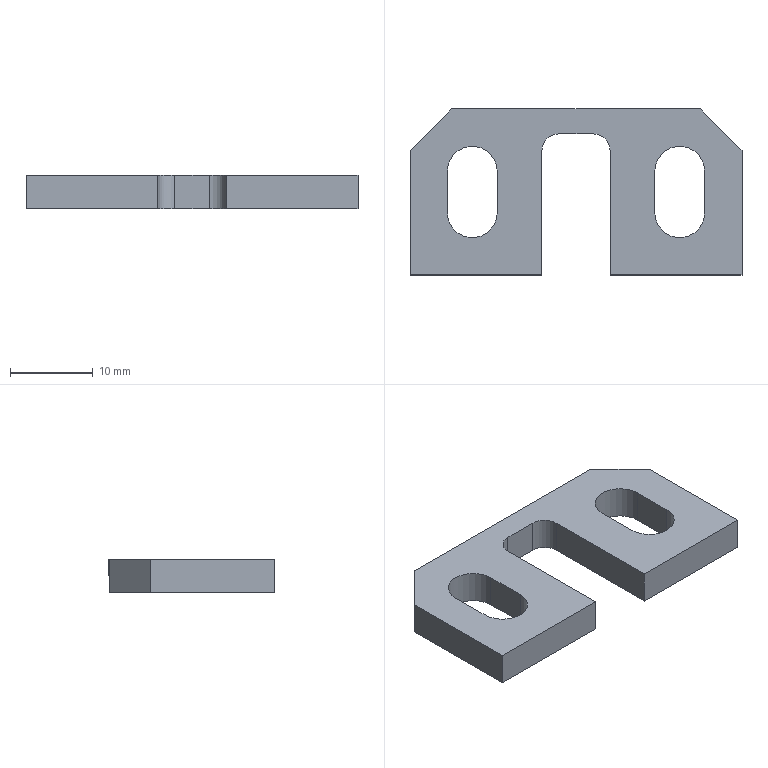Part | SolidWorks | features MirrorStock 1 | 1 solid | 22 faces | box 40 x 20 x 4 mm | volume 2083 mm3 | plane 16 | cylinder 6 | commonest cylinder face diameters 6 x4 4 x2
STEP:
#1=CARTESIAN_POINT('',(4.1,-10.,-4.));
#2=VERTEX_POINT('',#1);
#3=CARTESIAN_POINT('',(20.,-10.,-4.));
#4=VERTEX_POINT('',#3);
#5=CARTESIAN_POINT('',(-20.,-10.,-4.));
#6=DIRECTION('',(1.,0.,0.));
#7=VECTOR('',#6,1000.);
#8=LINE('',#5,#7);
#9=EDGE_CURVE('',#2,#4,#8,.T.);
#10=ORIENTED_EDGE('',*,*,#9,.T.);
#11=CARTESIAN_POINT('',(20.,-10.,0.));
#12=VERTEX_POINT('',#11);
#13=CARTESIAN_POINT('',(20.,-10.,-4.));
#14=DIRECTION('',(0.,0.,1.));
#15=VECTOR('',#14,1000.);
#16=LINE('',#13,#15);
#17=EDGE_CURVE('',#4,#12,#16,.T.);
#18=ORIENTED_EDGE('',*,*,#17,.T.);
#19=CARTESIAN_POINT('',(4.1,-10.,0.));
#20=VERTEX_POINT('',#19);
#21=CARTESIAN_POINT('',(-20.,-10.,0.));
#22=DIRECTION('',(1.,0.,0.));
#23=VECTOR('',#22,1000.);
#24=LINE('',#21,#23);
#25=EDGE_CURVE('',#20,#12,#24,.T.);
#26=ORIENTED_EDGE('',*,*,#25,.F.);
#27=CARTESIAN_POINT('',(4.1,-10.,-4.));
#28=DIRECTION('',(0.,0.,1.));
#29=VECTOR('',#28,1000.);
#30=LINE('',#27,#29);
#31=EDGE_CURVE('',#2,#20,#30,.T.);
#32=ORIENTED_EDGE('',*,*,#31,.F.);
#33=EDGE_LOOP('',(#10,#18,#26,#32));
#34=FACE_OUTER_BOUND('',#33,.T.);
#35=CARTESIAN_POINT('',(-20.,-10.,-4.));
#36=DIRECTION('',(0.,1.,0.));
#37=DIRECTION('',(-1.,0.,0.));
#38=AXIS2_PLACEMENT_3D('',#35,#36,#37);
#39=PLANE('',#38);
#40=ADVANCED_FACE('',(#34),#39,.F.);
#41=CARTESIAN_POINT('',(-20.,5.,-4.));
#42=VERTEX_POINT('',#41);
#43=CARTESIAN_POINT('',(-20.,-10.,-4.));
#44=VERTEX_POINT('',#43);
#45=CARTESIAN_POINT('',(-20.,10.,-4.));
#46=DIRECTION('',(0.,-1.,0.));
#47=VECTOR('',#46,1000.);
#48=LINE('',#45,#47);
#49=EDGE_CURVE('',#42,#44,#48,.T.);
#50=ORIENTED_EDGE('',*,*,#49,.T.);
#51=CARTESIAN_POINT('',(-20.,-10.,0.));
#52=VERTEX_POINT('',#51);
#53=CARTESIAN_POINT('',(-20.,-10.,-4.));
#54=DIRECTION('',(0.,0.,1.));
#55=VECTOR('',#54,1000.);
#56=LINE('',#53,#55);
#57=EDGE_CURVE('',#44,#52,#56,.T.);
#58=ORIENTED_EDGE('',*,*,#57,.T.);
#59=CARTESIAN_POINT('',(-20.,5.,0.));
#60=VERTEX_POINT('',#59);
#61=CARTESIAN_POINT('',(-20.,10.,0.));
#62=DIRECTION('',(0.,-1.,0.));
#63=VECTOR('',#62,1000.);
#64=LINE('',#61,#63);
#65=EDGE_CURVE('',#60,#52,#64,.T.);
#66=ORIENTED_EDGE('',*,*,#65,.F.);
#67=CARTESIAN_POINT('',(-20.,5.,-4.));
#68=DIRECTION('',(0.,0.,1.));
#69=VECTOR('',#68,1000.);
#70=LINE('',#67,#69);
#71=EDGE_CURVE('',#42,#60,#70,.T.);
#72=ORIENTED_EDGE('',*,*,#71,.F.);
#73=EDGE_LOOP('',(#50,#58,#66,#72));
#74=FACE_OUTER_BOUND('',#73,.T.);
#75=CARTESIAN_POINT('',(-20.,10.,-4.));
#76=DIRECTION('',(1.,0.,0.));
#77=DIRECTION('',(0.,0.,1.));
#78=AXIS2_PLACEMENT_3D('',#75,#76,#77);
#79=PLANE('',#78);
#80=ADVANCED_FACE('',(#74),#79,.F.);
#81=CARTESIAN_POINT('',(-4.1,-10.,0.));
#82=VERTEX_POINT('',#81);
#83=CARTESIAN_POINT('',(-20.,-10.,0.));
#84=DIRECTION('',(1.,0.,0.));
#85=VECTOR('',#84,1000.);
#86=LINE('',#83,#85);
#87=EDGE_CURVE('',#52,#82,#86,.T.);
#88=ORIENTED_EDGE('',*,*,#87,.F.);
#89=ORIENTED_EDGE('',*,*,#57,.F.);
#90=CARTESIAN_POINT('',(-4.1,-10.,-4.));
#91=VERTEX_POINT('',#90);
#92=CARTESIAN_POINT('',(-20.,-10.,-4.));
#93=DIRECTION('',(1.,0.,0.));
#94=VECTOR('',#93,1000.);
#95=LINE('',#92,#94);
#96=EDGE_CURVE('',#44,#91,#95,.T.);
#97=ORIENTED_EDGE('',*,*,#96,.T.);
#98=CARTESIAN_POINT('',(-4.1,-10.,-4.));
#99=DIRECTION('',(0.,0.,-1.));
#100=VECTOR('',#99,1000.);
#101=LINE('',#98,#100);
#102=EDGE_CURVE('',#82,#91,#101,.T.);
#103=ORIENTED_EDGE('',*,*,#102,.F.);
#104=EDGE_LOOP('',(#88,#89,#97,#103));
#105=FACE_OUTER_BOUND('',#104,.T.);
#106=CARTESIAN_POINT('',(-20.,-10.,-4.));
#107=DIRECTION('',(0.,1.,0.));
#108=DIRECTION('',(-1.,0.,0.));
#109=AXIS2_PLACEMENT_3D('',#106,#107,#108);
#110=PLANE('',#109);
#111=ADVANCED_FACE('',(#105),#110,.F.);
#112=CARTESIAN_POINT('',(20.,5.,0.));
#113=VERTEX_POINT('',#112);
#114=CARTESIAN_POINT('',(20.,10.,0.));
#115=DIRECTION('',(0.,1.,0.));
#116=VECTOR('',#115,1000.);
#117=LINE('',#114,#116);
#118=EDGE_CURVE('',#12,#113,#117,.T.);
#119=ORIENTED_EDGE('',*,*,#118,.F.);
#120=ORIENTED_EDGE('',*,*,#17,.F.);
#121=CARTESIAN_POINT('',(20.,5.,-4.));
#122=VERTEX_POINT('',#121);
#123=CARTESIAN_POINT('',(20.,10.,-4.));
#124=DIRECTION('',(0.,1.,0.));
#125=VECTOR('',#124,1000.);
#126=LINE('',#123,#125);
#127=EDGE_CURVE('',#4,#122,#126,.T.);
#128=ORIENTED_EDGE('',*,*,#127,.T.);
#129=CARTESIAN_POINT('',(20.,5.,-4.));
#130=DIRECTION('',(0.,0.,-1.));
#131=VECTOR('',#130,1000.);
#132=LINE('',#129,#131);
#133=EDGE_CURVE('',#113,#122,#132,.T.);
#134=ORIENTED_EDGE('',*,*,#133,.F.);
#135=EDGE_LOOP('',(#119,#120,#128,#134));
#136=FACE_OUTER_BOUND('',#135,.T.);
#137=CARTESIAN_POINT('',(20.,10.,-4.));
#138=DIRECTION('',(-1.,0.,0.));
#139=DIRECTION('',(0.,-1.,0.));
#140=AXIS2_PLACEMENT_3D('',#137,#138,#139);
#141=PLANE('',#140);
#142=ADVANCED_FACE('',(#136),#141,.F.);
#143=CARTESIAN_POINT('',(15.,10.,-4.));
#144=VERTEX_POINT('',#143);
#145=CARTESIAN_POINT('',(-15.,10.,-4.));
#146=VERTEX_POINT('',#145);
#147=CARTESIAN_POINT('',(-20.,10.,-4.));
#148=DIRECTION('',(-1.,0.,0.));
#149=VECTOR('',#148,1000.);
#150=LINE('',#147,#149);
#151=EDGE_CURVE('',#144,#146,#150,.T.);
#152=ORIENTED_EDGE('',*,*,#151,.T.);
#153=CARTESIAN_POINT('',(-15.,10.,0.));
#154=VERTEX_POINT('',#153);
#155=CARTESIAN_POINT('',(-15.,10.,-4.));
#156=DIRECTION('',(0.,0.,-1.));
#157=VECTOR('',#156,1000.);
#158=LINE('',#155,#157);
#159=EDGE_CURVE('',#154,#146,#158,.T.);
#160=ORIENTED_EDGE('',*,*,#159,.F.);
#161=CARTESIAN_POINT('',(15.,10.,0.));
#162=VERTEX_POINT('',#161);
#163=CARTESIAN_POINT('',(-20.,10.,0.));
#164=DIRECTION('',(-1.,0.,0.));
#165=VECTOR('',#164,1000.);
#166=LINE('',#163,#165);
#167=EDGE_CURVE('',#162,#154,#166,.T.);
#168=ORIENTED_EDGE('',*,*,#167,.F.);
#169=CARTESIAN_POINT('',(15.,10.,-4.));
#170=DIRECTION('',(0.,0.,1.));
#171=VECTOR('',#170,1000.);
#172=LINE('',#169,#171);
#173=EDGE_CURVE('',#144,#162,#172,.T.);
#174=ORIENTED_EDGE('',*,*,#173,.F.);
#175=EDGE_LOOP('',(#152,#160,#168,#174));
#176=FACE_OUTER_BOUND('',#175,.T.);
#177=CARTESIAN_POINT('',(-20.,10.,-4.));
#178=DIRECTION('',(0.,-1.,0.));
#179=DIRECTION('',(1.,0.,0.));
#180=AXIS2_PLACEMENT_3D('',#177,#178,#179);
#181=PLANE('',#180);
#182=ADVANCED_FACE('',(#176),#181,.F.);
#183=CARTESIAN_POINT('',(15.5,2.5,-4.));
#184=VERTEX_POINT('',#183);
#185=CARTESIAN_POINT('',(9.5,2.5,-4.));
#186=VERTEX_POINT('',#185);
#187=CARTESIAN_POINT('',(12.5,2.5,-4.));
#188=DIRECTION('',(0.,0.,1.));
#189=DIRECTION('',(1.,0.,0.));
#190=AXIS2_PLACEMENT_3D('',#187,#188,#189);
#191=CIRCLE('',#190,3.);
#192=EDGE_CURVE('',#184,#186,#191,.T.);
#193=ORIENTED_EDGE('',*,*,#192,.T.);
#194=CARTESIAN_POINT('',(9.5,-2.5,-4.));
#195=VERTEX_POINT('',#194);
#196=CARTESIAN_POINT('',(9.5,2.5,-4.));
#197=DIRECTION('',(0.,-1.,0.));
#198=VECTOR('',#197,1000.);
#199=LINE('',#196,#198);
#200=EDGE_CURVE('',#186,#195,#199,.T.);
#201=ORIENTED_EDGE('',*,*,#200,.T.);
#202=CARTESIAN_POINT('',(15.5,-2.5,-4.));
#203=VERTEX_POINT('',#202);
#204=CARTESIAN_POINT('',(12.5,-2.5,-4.));
#205=DIRECTION('',(0.,0.,1.));
#206=DIRECTION('',(1.,0.,0.));
#207=AXIS2_PLACEMENT_3D('',#204,#205,#206);
#208=CIRCLE('',#207,3.);
#209=EDGE_CURVE('',#195,#203,#208,.T.);
#210=ORIENTED_EDGE('',*,*,#209,.T.);
#211=CARTESIAN_POINT('',(15.5,2.5,-4.));
#212=DIRECTION('',(0.,1.,0.));
#213=VECTOR('',#212,1000.);
#214=LINE('',#211,#213);
#215=EDGE_CURVE('',#203,#184,#214,.T.);
#216=ORIENTED_EDGE('',*,*,#215,.T.);
#217=EDGE_LOOP('',(#193,#201,#210,#216));
#218=FACE_BOUND('',#217,.T.);
#219=CARTESIAN_POINT('',(-9.5,2.5,-4.));
#220=VERTEX_POINT('',#219);
#221=CARTESIAN_POINT('',(-15.5,2.5,-4.));
#222=VERTEX_POINT('',#221);
#223=CARTESIAN_POINT('',(-12.5,2.5,-4.));
#224=DIRECTION('',(0.,0.,1.));
#225=DIRECTION('',(1.,0.,0.));
#226=AXIS2_PLACEMENT_3D('',#223,#224,#225);
#227=CIRCLE('',#226,3.);
#228=EDGE_CURVE('',#220,#222,#227,.T.);
#229=ORIENTED_EDGE('',*,*,#228,.T.);
#230=CARTESIAN_POINT('',(-15.5,-2.5,-4.));
#231=VERTEX_POINT('',#230);
#232=CARTESIAN_POINT('',(-15.5,2.5,-4.));
#233=DIRECTION('',(0.,-1.,0.));
#234=VECTOR('',#233,1000.);
#235=LINE('',#232,#234);
#236=EDGE_CURVE('',#222,#231,#235,.T.);
#237=ORIENTED_EDGE('',*,*,#236,.T.);
#238=CARTESIAN_POINT('',(-9.5,-2.5,-4.));
#239=VERTEX_POINT('',#238);
#240=CARTESIAN_POINT('',(-12.5,-2.5,-4.));
#241=DIRECTION('',(0.,0.,1.));
#242=DIRECTION('',(1.,0.,0.));
#243=AXIS2_PLACEMENT_3D('',#240,#241,#242);
#244=CIRCLE('',#243,3.);
#245=EDGE_CURVE('',#231,#239,#244,.T.);
#246=ORIENTED_EDGE('',*,*,#245,.T.);
#247=CARTESIAN_POINT('',(-9.5,2.5,-4.));
#248=DIRECTION('',(0.,1.,0.));
#249=VECTOR('',#248,1000.);
#250=LINE('',#247,#249);
#251=EDGE_CURVE('',#239,#220,#250,.T.);
#252=ORIENTED_EDGE('',*,*,#251,.T.);
#253=EDGE_LOOP('',(#229,#237,#246,#252));
#254=FACE_BOUND('',#253,.T.);
#255=ORIENTED_EDGE('',*,*,#127,.F.);
#256=ORIENTED_EDGE('',*,*,#9,.F.);
#257=CARTESIAN_POINT('',(4.1,5.,-4.));
#258=VERTEX_POINT('',#257);
#259=CARTESIAN_POINT('',(4.1,7.,-4.));
#260=DIRECTION('',(0.,1.,0.));
#261=VECTOR('',#260,1000.);
#262=LINE('',#259,#261);
#263=EDGE_CURVE('',#2,#258,#262,.T.);
#264=ORIENTED_EDGE('',*,*,#263,.T.);
#265=CARTESIAN_POINT('',(2.1,7.,-4.));
#266=VERTEX_POINT('',#265);
#267=CARTESIAN_POINT('',(2.1,5.,-4.));
#268=DIRECTION('',(0.,0.,-1.));
#269=DIRECTION('',(1.,0.,0.));
#270=AXIS2_PLACEMENT_3D('',#267,#268,#269);
#271=CIRCLE('',#270,2.);
#272=EDGE_CURVE('',#266,#258,#271,.T.);
#273=ORIENTED_EDGE('',*,*,#272,.F.);
#274=CARTESIAN_POINT('',(-2.1,7.,-4.));
#275=VERTEX_POINT('',#274);
#276=CARTESIAN_POINT('',(-4.1,7.,-4.));
#277=DIRECTION('',(-1.,0.,0.));
#278=VECTOR('',#277,1000.);
#279=LINE('',#276,#278);
#280=EDGE_CURVE('',#266,#275,#279,.T.);
#281=ORIENTED_EDGE('',*,*,#280,.T.);
#282=CARTESIAN_POINT('',(-4.1,5.,-4.));
#283=VERTEX_POINT('',#282);
#284=CARTESIAN_POINT('',(-2.1,5.,-4.));
#285=DIRECTION('',(0.,0.,-1.));
#286=DIRECTION('',(1.,0.,0.));
#287=AXIS2_PLACEMENT_3D('',#284,#285,#286);
#288=CIRCLE('',#287,2.);
#289=EDGE_CURVE('',#283,#275,#288,.T.);
#290=ORIENTED_EDGE('',*,*,#289,.F.);
#291=CARTESIAN_POINT('',(-4.1,7.,-4.));
#292=DIRECTION('',(0.,-1.,0.));
#293=VECTOR('',#292,1000.);
#294=LINE('',#291,#293);
#295=EDGE_CURVE('',#283,#91,#294,.T.);
#296=ORIENTED_EDGE('',*,*,#295,.T.);
#297=ORIENTED_EDGE('',*,*,#96,.F.);
#298=ORIENTED_EDGE('',*,*,#49,.F.);
#299=CARTESIAN_POINT('',(-12.5,12.5,-4.));
#300=DIRECTION('',(-0.7071,-0.7071,0.));
#301=VECTOR('',#300,1000.);
#302=LINE('',#299,#301);
#303=EDGE_CURVE('',#146,#42,#302,.T.);
#304=ORIENTED_EDGE('',*,*,#303,.F.);
#305=ORIENTED_EDGE('',*,*,#151,.F.);
#306=CARTESIAN_POINT('',(12.5,12.5,-4.));
#307=DIRECTION('',(-0.7071,0.7071,0.));
#308=VECTOR('',#307,1000.);
#309=LINE('',#306,#308);
#310=EDGE_CURVE('',#122,#144,#309,.T.);
#311=ORIENTED_EDGE('',*,*,#310,.F.);
#312=EDGE_LOOP('',(#255,#256,#264,#273,#281,#290,#296,#297,#298,#304,#305,#311));
#313=FACE_OUTER_BOUND('',#312,.T.);
#314=CARTESIAN_POINT('',(0.,0.,-4.));
#315=DIRECTION('',(0.,0.,-1.));
#316=DIRECTION('',(1.,0.,0.));
#317=AXIS2_PLACEMENT_3D('',#314,#315,#316);
#318=PLANE('',#317);
#319=ADVANCED_FACE('',(#218,#254,#313),#318,.T.);
#320=CARTESIAN_POINT('',(9.5,-2.5,0.));
#321=VERTEX_POINT('',#320);
#322=CARTESIAN_POINT('',(15.5,-2.5,0.));
#323=VERTEX_POINT('',#322);
#324=CARTESIAN_POINT('',(12.5,-2.5,0.));
#325=DIRECTION('',(0.,0.,1.));
#326=DIRECTION('',(1.,0.,0.));
#327=AXIS2_PLACEMENT_3D('',#324,#325,#326);
#328=CIRCLE('',#327,3.);
#329=EDGE_CURVE('',#321,#323,#328,.T.);
#330=ORIENTED_EDGE('',*,*,#329,.F.);
#331=CARTESIAN_POINT('',(9.5,2.5,0.));
#332=VERTEX_POINT('',#331);
#333=CARTESIAN_POINT('',(9.5,2.5,0.));
#334=DIRECTION('',(0.,-1.,0.));
#335=VECTOR('',#334,1000.);
#336=LINE('',#333,#335);
#337=EDGE_CURVE('',#332,#321,#336,.T.);
#338=ORIENTED_EDGE('',*,*,#337,.F.);
#339=CARTESIAN_POINT('',(15.5,2.5,0.));
#340=VERTEX_POINT('',#339);
#341=CARTESIAN_POINT('',(12.5,2.5,0.));
#342=DIRECTION('',(0.,0.,1.));
#343=DIRECTION('',(1.,0.,0.));
#344=AXIS2_PLACEMENT_3D('',#341,#342,#343);
#345=CIRCLE('',#344,3.);
#346=EDGE_CURVE('',#340,#332,#345,.T.);
#347=ORIENTED_EDGE('',*,*,#346,.F.);
#348=CARTESIAN_POINT('',(15.5,2.5,0.));
#349=DIRECTION('',(0.,1.,0.));
#350=VECTOR('',#349,1000.);
#351=LINE('',#348,#350);
#352=EDGE_CURVE('',#323,#340,#351,.T.);
#353=ORIENTED_EDGE('',*,*,#352,.F.);
#354=EDGE_LOOP('',(#330,#338,#347,#353));
#355=FACE_BOUND('',#354,.T.);
#356=CARTESIAN_POINT('',(-15.5,-2.5,0.));
#357=VERTEX_POINT('',#356);
#358=CARTESIAN_POINT('',(-9.5,-2.5,0.));
#359=VERTEX_POINT('',#358);
#360=CARTESIAN_POINT('',(-12.5,-2.5,0.));
#361=DIRECTION('',(0.,0.,1.));
#362=DIRECTION('',(1.,0.,0.));
#363=AXIS2_PLACEMENT_3D('',#360,#361,#362);
#364=CIRCLE('',#363,3.);
#365=EDGE_CURVE('',#357,#359,#364,.T.);
#366=ORIENTED_EDGE('',*,*,#365,.F.);
#367=CARTESIAN_POINT('',(-15.5,2.5,0.));
#368=VERTEX_POINT('',#367);
#369=CARTESIAN_POINT('',(-15.5,2.5,0.));
#370=DIRECTION('',(0.,-1.,0.));
#371=VECTOR('',#370,1000.);
#372=LINE('',#369,#371);
#373=EDGE_CURVE('',#368,#357,#372,.T.);
#374=ORIENTED_EDGE('',*,*,#373,.F.);
#375=CARTESIAN_POINT('',(-9.5,2.5,0.));
#376=VERTEX_POINT('',#375);
#377=CARTESIAN_POINT('',(-12.5,2.5,0.));
#378=DIRECTION('',(0.,0.,1.));
#379=DIRECTION('',(1.,0.,0.));
#380=AXIS2_PLACEMENT_3D('',#377,#378,#379);
#381=CIRCLE('',#380,3.);
#382=EDGE_CURVE('',#376,#368,#381,.T.);
#383=ORIENTED_EDGE('',*,*,#382,.F.);
#384=CARTESIAN_POINT('',(-9.5,2.5,0.));
#385=DIRECTION('',(0.,1.,0.));
#386=VECTOR('',#385,1000.);
#387=LINE('',#384,#386);
#388=EDGE_CURVE('',#359,#376,#387,.T.);
#389=ORIENTED_EDGE('',*,*,#388,.F.);
#390=EDGE_LOOP('',(#366,#374,#383,#389));
#391=FACE_BOUND('',#390,.T.);
#392=ORIENTED_EDGE('',*,*,#167,.T.);
#393=CARTESIAN_POINT('',(-20.,5.,0.));
#394=DIRECTION('',(0.7071,0.7071,0.));
#395=VECTOR('',#394,1000.);
#396=LINE('',#393,#395);
#397=EDGE_CURVE('',#60,#154,#396,.T.);
#398=ORIENTED_EDGE('',*,*,#397,.F.);
#399=ORIENTED_EDGE('',*,*,#65,.T.);
#400=ORIENTED_EDGE('',*,*,#87,.T.);
#401=CARTESIAN_POINT('',(-4.1,5.,0.));
#402=VERTEX_POINT('',#401);
#403=CARTESIAN_POINT('',(-4.1,7.,0.));
#404=DIRECTION('',(0.,-1.,0.));
#405=VECTOR('',#404,1000.);
#406=LINE('',#403,#405);
#407=EDGE_CURVE('',#402,#82,#406,.T.);
#408=ORIENTED_EDGE('',*,*,#407,.F.);
#409=CARTESIAN_POINT('',(-2.1,7.,0.));
#410=VERTEX_POINT('',#409);
#411=CARTESIAN_POINT('',(-2.1,5.,0.));
#412=DIRECTION('',(0.,0.,1.));
#413=DIRECTION('',(1.,0.,0.));
#414=AXIS2_PLACEMENT_3D('',#411,#412,#413);
#415=CIRCLE('',#414,2.);
#416=EDGE_CURVE('',#410,#402,#415,.T.);
#417=ORIENTED_EDGE('',*,*,#416,.F.);
#418=CARTESIAN_POINT('',(2.1,7.,0.));
#419=VERTEX_POINT('',#418);
#420=CARTESIAN_POINT('',(-4.1,7.,0.));
#421=DIRECTION('',(-1.,0.,0.));
#422=VECTOR('',#421,1000.);
#423=LINE('',#420,#422);
#424=EDGE_CURVE('',#419,#410,#423,.T.);
#425=ORIENTED_EDGE('',*,*,#424,.F.);
#426=CARTESIAN_POINT('',(4.1,5.,0.));
#427=VERTEX_POINT('',#426);
#428=CARTESIAN_POINT('',(2.1,5.,0.));
#429=DIRECTION('',(0.,0.,1.));
#430=DIRECTION('',(1.,0.,0.));
#431=AXIS2_PLACEMENT_3D('',#428,#429,#430);
#432=CIRCLE('',#431,2.);
#433=EDGE_CURVE('',#427,#419,#432,.T.);
#434=ORIENTED_EDGE('',*,*,#433,.F.);
#435=CARTESIAN_POINT('',(4.1,0.,0.));
#436=DIRECTION('',(0.,1.,0.));
#437=VECTOR('',#436,1000.);
#438=LINE('',#435,#437);
#439=EDGE_CURVE('',#20,#427,#438,.T.);
#440=ORIENTED_EDGE('',*,*,#439,.F.);
#441=ORIENTED_EDGE('',*,*,#25,.T.);
#442=ORIENTED_EDGE('',*,*,#118,.T.);
#443=CARTESIAN_POINT('',(15.,10.,0.));
#444=DIRECTION('',(0.7071,-0.7071,0.));
#445=VECTOR('',#444,1000.);
#446=LINE('',#443,#445);
#447=EDGE_CURVE('',#162,#113,#446,.T.);
#448=ORIENTED_EDGE('',*,*,#447,.F.);
#449=EDGE_LOOP('',(#392,#398,#399,#400,#408,#417,#425,#434,#440,#441,#442,#448));
#450=FACE_OUTER_BOUND('',#449,.T.);
#451=CARTESIAN_POINT('',(0.,0.,0.));
#452=DIRECTION('',(0.,0.,-1.));
#453=DIRECTION('',(1.,0.,0.));
#454=AXIS2_PLACEMENT_3D('',#451,#452,#453);
#455=PLANE('',#454);
#456=ADVANCED_FACE('',(#355,#391,#450),#455,.F.);
#457=ORIENTED_EDGE('',*,*,#263,.F.);
#458=ORIENTED_EDGE('',*,*,#31,.T.);
#459=ORIENTED_EDGE('',*,*,#439,.T.);
#460=CARTESIAN_POINT('',(4.1,5.,0.));
#461=DIRECTION('',(0.,0.,1.));
#462=VECTOR('',#461,1000.);
#463=LINE('',#460,#462);
#464=EDGE_CURVE('',#258,#427,#463,.T.);
#465=ORIENTED_EDGE('',*,*,#464,.F.);
#466=EDGE_LOOP('',(#457,#458,#459,#465));
#467=FACE_OUTER_BOUND('',#466,.T.);
#468=CARTESIAN_POINT('',(4.1,7.,0.));
#469=DIRECTION('',(1.,0.,0.));
#470=DIRECTION('',(0.,1.,0.));
#471=AXIS2_PLACEMENT_3D('',#468,#469,#470);
#472=PLANE('',#471);
#473=ADVANCED_FACE('',(#467),#472,.F.);
#474=ORIENTED_EDGE('',*,*,#407,.T.);
#475=ORIENTED_EDGE('',*,*,#102,.T.);
#476=ORIENTED_EDGE('',*,*,#295,.F.);
#477=CARTESIAN_POINT('',(-4.1,5.,-4.));
#478=DIRECTION('',(0.,0.,-1.));
#479=VECTOR('',#478,1000.);
#480=LINE('',#477,#479);
#481=EDGE_CURVE('',#402,#283,#480,.T.);
#482=ORIENTED_EDGE('',*,*,#481,.F.);
#483=EDGE_LOOP('',(#474,#475,#476,#482));
#484=FACE_OUTER_BOUND('',#483,.T.);
#485=CARTESIAN_POINT('',(-4.1,7.,0.));
#486=DIRECTION('',(-1.,0.,0.));
#487=DIRECTION('',(0.,-1.,0.));
#488=AXIS2_PLACEMENT_3D('',#485,#486,#487);
#489=PLANE('',#488);
#490=ADVANCED_FACE('',(#484),#489,.F.);
#491=ORIENTED_EDGE('',*,*,#424,.T.);
#492=CARTESIAN_POINT('',(-2.1,7.,0.));
#493=DIRECTION('',(0.,0.,1.));
#494=VECTOR('',#493,1000.);
#495=LINE('',#492,#494);
#496=EDGE_CURVE('',#275,#410,#495,.T.);
#497=ORIENTED_EDGE('',*,*,#496,.F.);
#498=ORIENTED_EDGE('',*,*,#280,.F.);
#499=CARTESIAN_POINT('',(2.1,7.,-4.));
#500=DIRECTION('',(0.,0.,-1.));
#501=VECTOR('',#500,1000.);
#502=LINE('',#499,#501);
#503=EDGE_CURVE('',#419,#266,#502,.T.);
#504=ORIENTED_EDGE('',*,*,#503,.F.);
#505=EDGE_LOOP('',(#491,#497,#498,#504));
#506=FACE_OUTER_BOUND('',#505,.T.);
#507=CARTESIAN_POINT('',(-4.1,7.,0.));
#508=DIRECTION('',(0.,1.,0.));
#509=DIRECTION('',(-1.,0.,0.));
#510=AXIS2_PLACEMENT_3D('',#507,#508,#509);
#511=PLANE('',#510);
#512=ADVANCED_FACE('',(#506),#511,.F.);
#513=ORIENTED_EDGE('',*,*,#310,.T.);
#514=ORIENTED_EDGE('',*,*,#173,.T.);
#515=ORIENTED_EDGE('',*,*,#447,.T.);
#516=ORIENTED_EDGE('',*,*,#133,.T.);
#517=EDGE_LOOP('',(#513,#514,#515,#516));
#518=FACE_OUTER_BOUND('',#517,.T.);
#519=CARTESIAN_POINT('',(15.,10.,-4.));
#520=DIRECTION('',(-0.7071,-0.7071,0.));
#521=DIRECTION('',(0.,0.,1.));
#522=AXIS2_PLACEMENT_3D('',#519,#520,#521);
#523=PLANE('',#522);
#524=ADVANCED_FACE('',(#518),#523,.F.);
#525=ORIENTED_EDGE('',*,*,#303,.T.);
#526=ORIENTED_EDGE('',*,*,#71,.T.);
#527=ORIENTED_EDGE('',*,*,#397,.T.);
#528=ORIENTED_EDGE('',*,*,#159,.T.);
#529=EDGE_LOOP('',(#525,#526,#527,#528));
#530=FACE_OUTER_BOUND('',#529,.T.);
#531=CARTESIAN_POINT('',(-20.,5.,-4.));
#532=DIRECTION('',(0.7071,-0.7071,0.));
#533=DIRECTION('',(0.,0.,1.));
#534=AXIS2_PLACEMENT_3D('',#531,#532,#533);
#535=PLANE('',#534);
#536=ADVANCED_FACE('',(#530),#535,.F.);
#537=ORIENTED_EDGE('',*,*,#251,.F.);
#538=CARTESIAN_POINT('',(-9.5,-2.5,0.));
#539=DIRECTION('',(0.,0.,-1.));
#540=VECTOR('',#539,1000.);
#541=LINE('',#538,#540);
#542=EDGE_CURVE('',#359,#239,#541,.T.);
#543=ORIENTED_EDGE('',*,*,#542,.F.);
#544=ORIENTED_EDGE('',*,*,#388,.T.);
#545=CARTESIAN_POINT('',(-9.5,2.5,0.));
#546=DIRECTION('',(0.,0.,-1.));
#547=VECTOR('',#546,1000.);
#548=LINE('',#545,#547);
#549=EDGE_CURVE('',#376,#220,#548,.T.);
#550=ORIENTED_EDGE('',*,*,#549,.T.);
#551=EDGE_LOOP('',(#537,#543,#544,#550));
#552=FACE_OUTER_BOUND('',#551,.T.);
#553=CARTESIAN_POINT('',(-9.5,2.5,0.));
#554=DIRECTION('',(1.,0.,0.));
#555=DIRECTION('',(0.,1.,0.));
#556=AXIS2_PLACEMENT_3D('',#553,#554,#555);
#557=PLANE('',#556);
#558=ADVANCED_FACE('',(#552),#557,.F.);
#559=ORIENTED_EDGE('',*,*,#236,.F.);
#560=CARTESIAN_POINT('',(-15.5,2.5,0.));
#561=DIRECTION('',(0.,0.,-1.));
#562=VECTOR('',#561,1000.);
#563=LINE('',#560,#562);
#564=EDGE_CURVE('',#368,#222,#563,.T.);
#565=ORIENTED_EDGE('',*,*,#564,.F.);
#566=ORIENTED_EDGE('',*,*,#373,.T.);
#567=CARTESIAN_POINT('',(-15.5,-2.5,0.));
#568=DIRECTION('',(0.,0.,-1.));
#569=VECTOR('',#568,1000.);
#570=LINE('',#567,#569);
#571=EDGE_CURVE('',#357,#231,#570,.T.);
#572=ORIENTED_EDGE('',*,*,#571,.T.);
#573=EDGE_LOOP('',(#559,#565,#566,#572));
#574=FACE_OUTER_BOUND('',#573,.T.);
#575=CARTESIAN_POINT('',(-15.5,2.5,0.));
#576=DIRECTION('',(-1.,0.,0.));
#577=DIRECTION('',(0.,0.,-1.));
#578=AXIS2_PLACEMENT_3D('',#575,#576,#577);
#579=PLANE('',#578);
#580=ADVANCED_FACE('',(#574),#579,.F.);
#581=ORIENTED_EDGE('',*,*,#228,.F.);
#582=ORIENTED_EDGE('',*,*,#549,.F.);
#583=ORIENTED_EDGE('',*,*,#382,.T.);
#584=ORIENTED_EDGE('',*,*,#564,.T.);
#585=EDGE_LOOP('',(#581,#582,#583,#584));
#586=FACE_OUTER_BOUND('',#585,.T.);
#587=CARTESIAN_POINT('',(-12.5,2.5,0.));
#588=DIRECTION('',(0.,0.,-1.));
#589=DIRECTION('',(1.,0.,0.));
#590=AXIS2_PLACEMENT_3D('',#587,#588,#589);
#591=CYLINDRICAL_SURFACE('',#590,3.);
#592=ADVANCED_FACE('',(#586),#591,.F.);
#593=ORIENTED_EDGE('',*,*,#245,.F.);
#594=ORIENTED_EDGE('',*,*,#571,.F.);
#595=ORIENTED_EDGE('',*,*,#365,.T.);
#596=ORIENTED_EDGE('',*,*,#542,.T.);
#597=EDGE_LOOP('',(#593,#594,#595,#596));
#598=FACE_OUTER_BOUND('',#597,.T.);
#599=CARTESIAN_POINT('',(-12.5,-2.5,0.));
#600=DIRECTION('',(0.,0.,-1.));
#601=DIRECTION('',(1.,0.,0.));
#602=AXIS2_PLACEMENT_3D('',#599,#600,#601);
#603=CYLINDRICAL_SURFACE('',#602,3.);
#604=ADVANCED_FACE('',(#598),#603,.F.);
#605=ORIENTED_EDGE('',*,*,#215,.F.);
#606=CARTESIAN_POINT('',(15.5,-2.5,0.));
#607=DIRECTION('',(0.,0.,-1.));
#608=VECTOR('',#607,1000.);
#609=LINE('',#606,#608);
#610=EDGE_CURVE('',#323,#203,#609,.T.);
#611=ORIENTED_EDGE('',*,*,#610,.F.);
#612=ORIENTED_EDGE('',*,*,#352,.T.);
#613=CARTESIAN_POINT('',(15.5,2.5,0.));
#614=DIRECTION('',(0.,0.,-1.));
#615=VECTOR('',#614,1000.);
#616=LINE('',#613,#615);
#617=EDGE_CURVE('',#340,#184,#616,.T.);
#618=ORIENTED_EDGE('',*,*,#617,.T.);
#619=EDGE_LOOP('',(#605,#611,#612,#618));
#620=FACE_OUTER_BOUND('',#619,.T.);
#621=CARTESIAN_POINT('',(15.5,2.5,0.));
#622=DIRECTION('',(1.,0.,0.));
#623=DIRECTION('',(0.,1.,0.));
#624=AXIS2_PLACEMENT_3D('',#621,#622,#623);
#625=PLANE('',#624);
#626=ADVANCED_FACE('',(#620),#625,.F.);
#627=ORIENTED_EDGE('',*,*,#200,.F.);
#628=CARTESIAN_POINT('',(9.5,2.5,0.));
#629=DIRECTION('',(0.,0.,-1.));
#630=VECTOR('',#629,1000.);
#631=LINE('',#628,#630);
#632=EDGE_CURVE('',#332,#186,#631,.T.);
#633=ORIENTED_EDGE('',*,*,#632,.F.);
#634=ORIENTED_EDGE('',*,*,#337,.T.);
#635=CARTESIAN_POINT('',(9.5,-2.5,0.));
#636=DIRECTION('',(0.,0.,-1.));
#637=VECTOR('',#636,1000.);
#638=LINE('',#635,#637);
#639=EDGE_CURVE('',#321,#195,#638,.T.);
#640=ORIENTED_EDGE('',*,*,#639,.T.);
#641=EDGE_LOOP('',(#627,#633,#634,#640));
#642=FACE_OUTER_BOUND('',#641,.T.);
#643=CARTESIAN_POINT('',(9.5,2.5,0.));
#644=DIRECTION('',(-1.,0.,0.));
#645=DIRECTION('',(0.,0.,-1.));
#646=AXIS2_PLACEMENT_3D('',#643,#644,#645);
#647=PLANE('',#646);
#648=ADVANCED_FACE('',(#642),#647,.F.);
#649=ORIENTED_EDGE('',*,*,#192,.F.);
#650=ORIENTED_EDGE('',*,*,#617,.F.);
#651=ORIENTED_EDGE('',*,*,#346,.T.);
#652=ORIENTED_EDGE('',*,*,#632,.T.);
#653=EDGE_LOOP('',(#649,#650,#651,#652));
#654=FACE_OUTER_BOUND('',#653,.T.);
#655=CARTESIAN_POINT('',(12.5,2.5,0.));
#656=DIRECTION('',(0.,0.,-1.));
#657=DIRECTION('',(1.,0.,0.));
#658=AXIS2_PLACEMENT_3D('',#655,#656,#657);
#659=CYLINDRICAL_SURFACE('',#658,3.);
#660=ADVANCED_FACE('',(#654),#659,.F.);
#661=ORIENTED_EDGE('',*,*,#209,.F.);
#662=ORIENTED_EDGE('',*,*,#639,.F.);
#663=ORIENTED_EDGE('',*,*,#329,.T.);
#664=ORIENTED_EDGE('',*,*,#610,.T.);
#665=EDGE_LOOP('',(#661,#662,#663,#664));
#666=FACE_OUTER_BOUND('',#665,.T.);
#667=CARTESIAN_POINT('',(12.5,-2.5,0.));
#668=DIRECTION('',(0.,0.,-1.));
#669=DIRECTION('',(1.,0.,0.));
#670=AXIS2_PLACEMENT_3D('',#667,#668,#669);
#671=CYLINDRICAL_SURFACE('',#670,3.);
#672=ADVANCED_FACE('',(#666),#671,.F.);
#673=ORIENTED_EDGE('',*,*,#433,.T.);
#674=ORIENTED_EDGE('',*,*,#503,.T.);
#675=ORIENTED_EDGE('',*,*,#272,.T.);
#676=ORIENTED_EDGE('',*,*,#464,.T.);
#677=EDGE_LOOP('',(#673,#674,#675,#676));
#678=FACE_OUTER_BOUND('',#677,.T.);
#679=CARTESIAN_POINT('',(2.1,5.,0.));
#680=DIRECTION('',(0.,0.,1.));
#681=DIRECTION('',(-1.,0.,0.));
#682=AXIS2_PLACEMENT_3D('',#679,#680,#681);
#683=CYLINDRICAL_SURFACE('',#682,2.);
#684=ADVANCED_FACE('',(#678),#683,.F.);
#685=ORIENTED_EDGE('',*,*,#416,.T.);
#686=ORIENTED_EDGE('',*,*,#481,.T.);
#687=ORIENTED_EDGE('',*,*,#289,.T.);
#688=ORIENTED_EDGE('',*,*,#496,.T.);
#689=EDGE_LOOP('',(#685,#686,#687,#688));
#690=FACE_OUTER_BOUND('',#689,.T.);
#691=CARTESIAN_POINT('',(-2.1,5.,0.));
#692=DIRECTION('',(0.,0.,1.));
#693=DIRECTION('',(-1.,0.,0.));
#694=AXIS2_PLACEMENT_3D('',#691,#692,#693);
#695=CYLINDRICAL_SURFACE('',#694,2.);
#696=ADVANCED_FACE('',(#690),#695,.F.);
#697=CLOSED_SHELL('',(#40,#80,#111,#142,#182,#319,#456,#473,#490,#512,#524,#536,#558,#580,#592,#604,#626,#648,#660,#672,#684,#696));
#698=MANIFOLD_SOLID_BREP('',#697);
#699=CARTESIAN_POINT('',(0.,0.,0.));
#700=DIRECTION('',(0.,0.,1.));
#701=DIRECTION('',(1.,0.,0.));
#702=AXIS2_PLACEMENT_3D('',#699,#700,#701);
#703=(LENGTH_UNIT()NAMED_UNIT(*)SI_UNIT(.MILLI.,.METRE.));
#704=UNCERTAINTY_MEASURE_WITH_UNIT(LENGTH_MEASURE(0.00001),#703,'','');
#705=(NAMED_UNIT(*)PLANE_ANGLE_UNIT()SI_UNIT($,.RADIAN.));
#706=(NAMED_UNIT(*)SI_UNIT($,.STERADIAN.)SOLID_ANGLE_UNIT());
#707=(GEOMETRIC_REPRESENTATION_CONTEXT(3)GLOBAL_UNCERTAINTY_ASSIGNED_CONTEXT((#704))GLOBAL_UNIT_ASSIGNED_CONTEXT((#703,#705,#706))REPRESENTATION_CONTEXT('',''));
#708=ADVANCED_BREP_SHAPE_REPRESENTATION('',(#698,#702),#707);